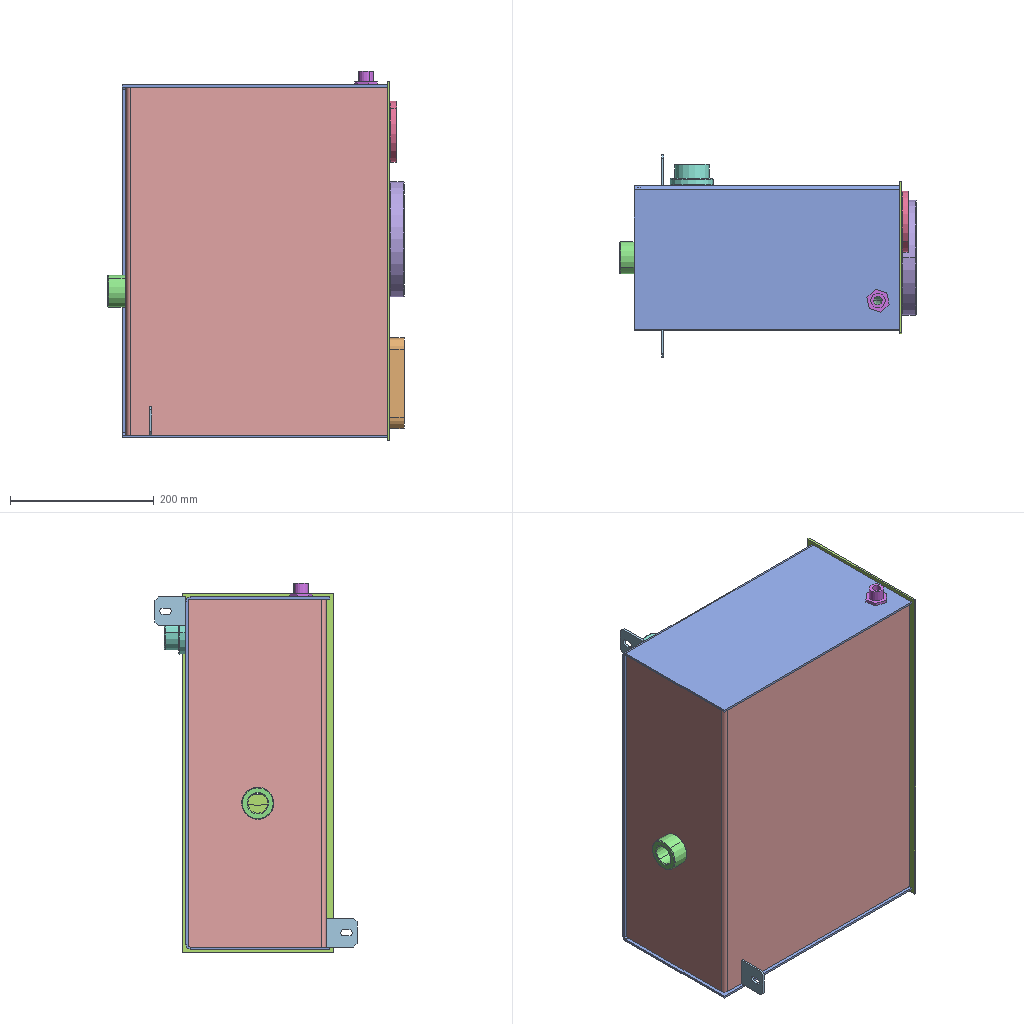Assembly | SolidWorks | 12 different items | 13 placed | box 412 x 281 x 514 mm
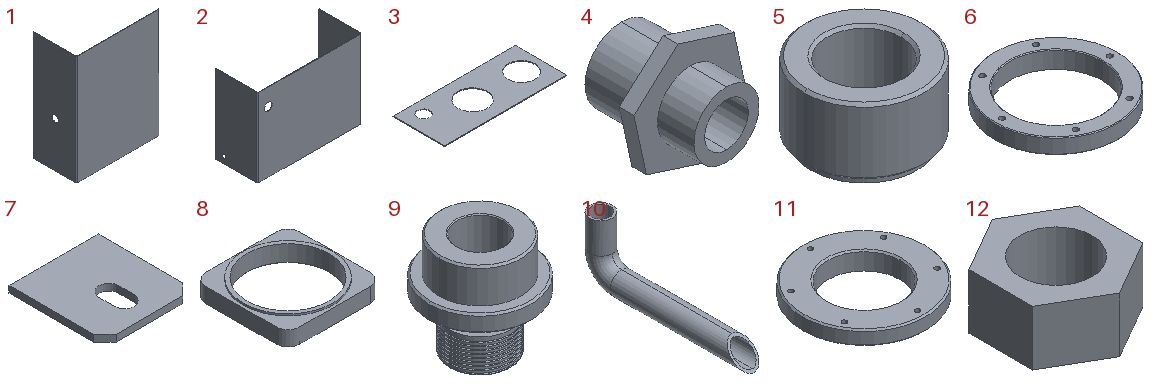Parts list (item | quantity | size | volume | features):
1 | x1 | 364 x 192 x 484 mm | 798031 mm3 | features Cut 1, FlatPattern 1, SMBaseFlange 1, SheetMetal 1
2 | x1 | 490 x 200 x 369 mm | 969574 mm3 | features Cut 3, FlatPattern 1, SMBaseFlange 1, SheetMetal 1
3 | x1 | 500 x 210 x 3 mm | 246670 mm3 | features Cut 1, Extrusion 1
4 | x1 | 31.039 x 29 x 31.865 mm | 6770 mm3 | features ICE 2, Extrusion 1
5 | x1 | 45 x 45 x 27.5 mm | 25785 mm3 | features 3DProfileFeature 1, Chamfer 1, Extrusion 1, HoleWzd 1, ICE 1
6 | x1 | 160 x 160 x 22.5 mm | 187073 mm3 | features 3DProfileFeature 1, Chamfer 1, Extrusion 1, HoleWzd 1, ICE 1
7 | x2 | 40 x 43 x 3 mm | 4705 mm3 | features Extrusion 1
8 | x1 | 126 x 126 x 22.5 mm | 124484 mm3 | features 3DProfileFeature 1, Chamfer 1, Extrusion 1, HoleWzd 1, ICE 1
9 | x1 | 60 x 60 x 60 mm | 59029 mm3 | -
10 | x1 | 22 x 161 x 61 mm | 22672 mm3 | features ICE 1, Sweep 1
11 | x1 | 85 x 85 x 12.5 mm | 41153 mm3 | features 3DProfileFeature 1, Chamfer 1, Extrusion 1, HoleWzd 1, ICE 1
12 | x1 | 16 x 18.475 x 8 mm | 1094 mm3 | features Extrusion 1
Mates (type | each side: item.copy, entity, surface, feature):
Coincident | 1.1 face plane Base-Flange1 | 2.1 face plane Base-Flange1 | 2 times
DistanceDim | 1.1 face plane Base-Flange1 | 2.1 face plane Base-Flange1
Coincident | 2.1 face plane Base-Flange1 | 3.1 face plane Boss-Extrude1
DistanceDim | 3.1 face plane Boss-Extrude1 | 2.1 face plane Base-Flange1 | 2 times
Coincident | 2.1 face plane Base-Flange1 | 9.1 face plane Boss-Extrude2
Concentric | 2.1 edge | 9.1 edge
Coincident | 3.1 face plane Boss-Extrude1 | 6.1 face plane Boss-Extrude1
Concentric | 3.1 edge | 6.1 edge
Coincident | 3.1 face plane Boss-Extrude1 | 8.1 face plane Boss-Extrude1
Concentric | 3.1 edge | 8.1 edge
Coincident | 1.1 face plane Base-Flange1 | 5.1 face plane Boss-Extrude2
Concentric | 1.1 edge | 5.1 edge
Coincident | 3.1 face plane Boss-Extrude1 | 11.1 face plane Boss-Extrude1
Concentric | 3.1 edge | 11.1 edge
DistanceDim | 2.1 face plane Base-Flange1 | 7.1 face plane Boss-Extrude1
Coincident | 1.1 face plane Base-Flange1 | 7.1 face plane Boss-Extrude1
Coincident | 2.1 face plane Base-Flange1 | 7.1 face plane Boss-Extrude1
Coincident | 7.1 face plane Boss-Extrude1 | 7.2 face plane Boss-Extrude1
Coincident | 2.1 face plane Base-Flange1 | 7.2 face plane Boss-Extrude1 | 2 times
Concentric | 2.1 edge | assembly edge
Coincident | 2.1 face plane Base-Flange1 | assembly face
Coincident | 2.1 face plane Base-Flange1 | 10.1 face plane Sweep1
Concentric | 2.1 edge | 10.1 edge
Coincident | 2.1 face plane Base-Flange1 | 4.1 face plane Boss-Extrude2
Concentric | 2.1 edge | 4.1 edge
Concentric | 2.1 edge | 12.1 edge
Coincident | 2.1 face plane Base-Flange1 | 12.1 face plane Boss-Extrude1